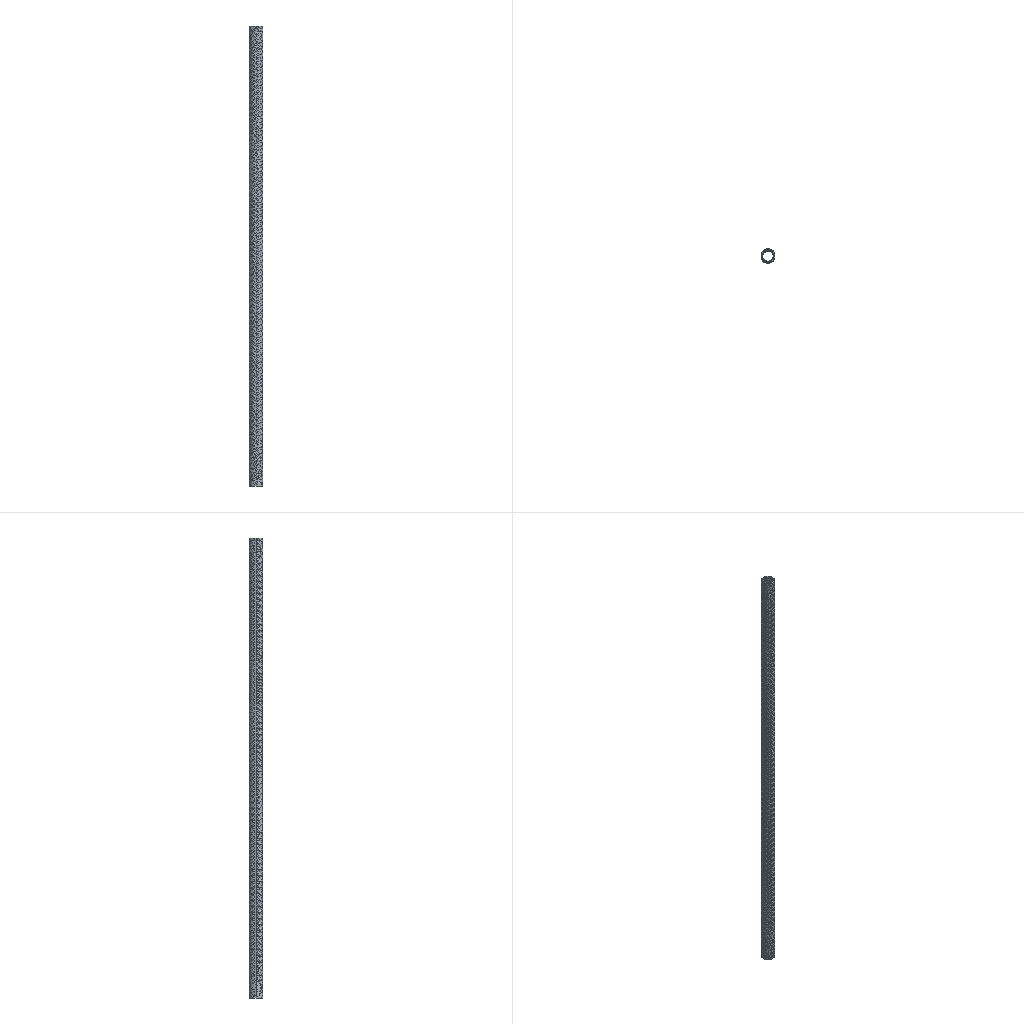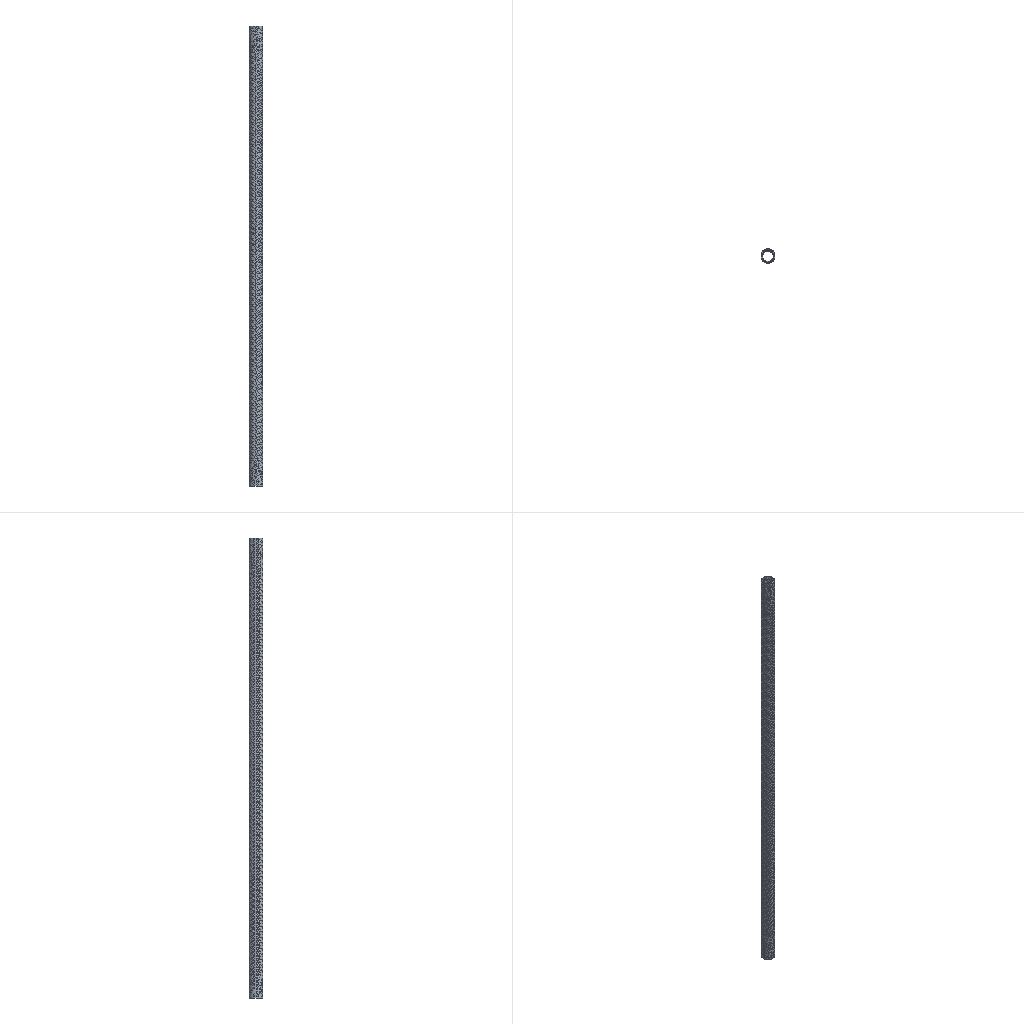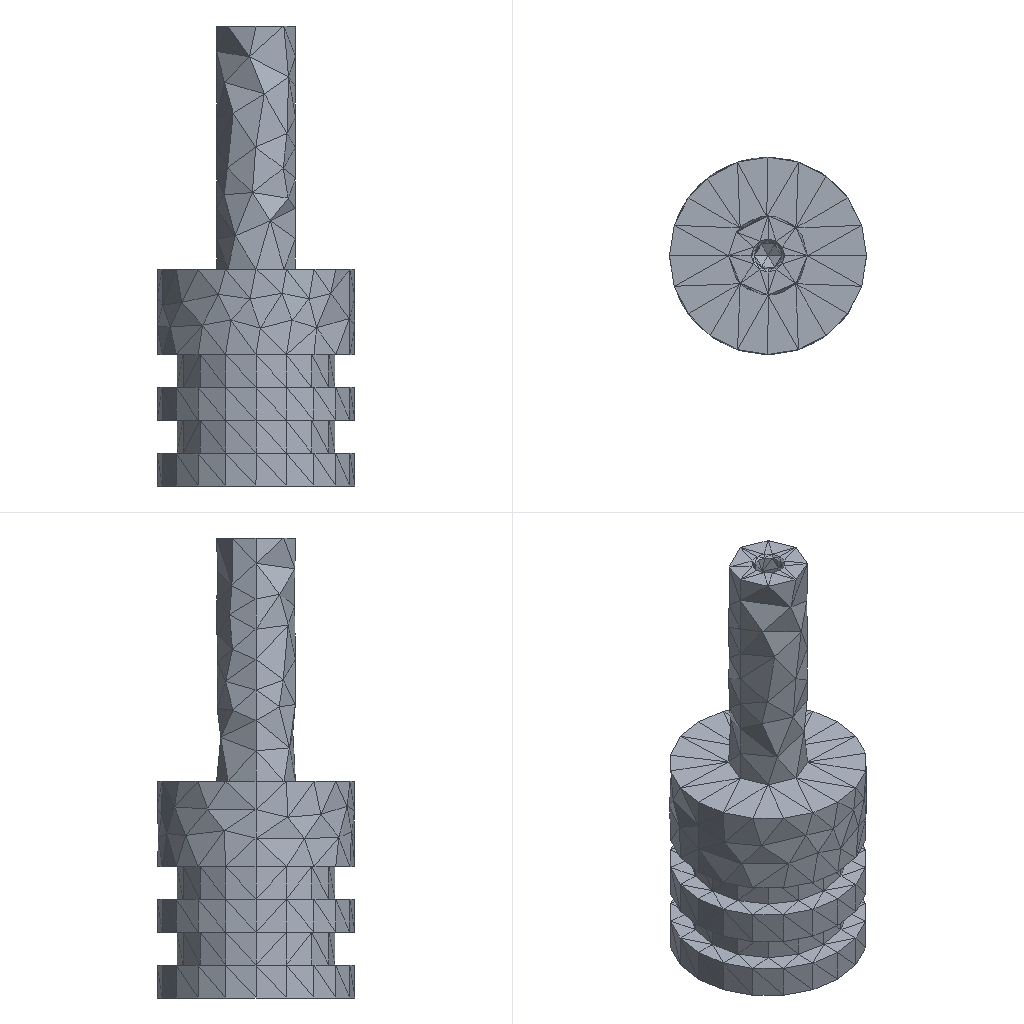Simulation study | ansys workbench
Set-up summary:
category,name,step,type,value,unit,region
solver,ansys_mapdl
solver,version,,,22.1
solver,version,,,22.1
solver,version,,,22.1
solver,version,,,22.1
solver,version,,,22.1
solver,version,,,22.1
units,MPA,,stated
analysis,deck1,,static,static
load_step,requested,,,1
analysis,nlgeom,,,False
mesh,nodes,,,29678
mesh,elements,,,19517
element_type,ANSYS 187 (type 1),,solid,14973
element_type,ANSYS 174 (type 2),,contact,4544
element_type,ANSYS 170 (type 3),,target,0
load,load commands in deck,,count,3
bc,support commands in deck,,count,1
named_set,_FIXEDSU,,component
analysis,deck2,,static,static
load_step,requested,,,1
analysis,nlgeom,,,False
mesh,nodes,,,24907
mesh,elements,,,16520
element_type,ANSYS 187 (type 1),,solid,12612
element_type,ANSYS 174 (type 2),,contact,3908
element_type,ANSYS 170 (type 3),,target,0
load,load commands in deck,,count,3
bc,support commands in deck,,count,1
named_set,_FIXEDSU,,component
analysis,deck3,,static,static
load_step,requested,,,1
analysis,nlgeom,,,False
mesh,nodes,,,2582
mesh,elements,,,1527
element_type,ANSYS 187 (type 1),,solid,1357
element_type,ANSYS 174 (type 2),,contact,170
element_type,ANSYS 170 (type 3),,target,0
load,load commands in deck,,count,3
bc,support commands in deck,,count,1
named_set,_FIXEDSU,,component
analysis,deck4,,static,static
load_step,requested,,,1
analysis,nlgeom,,,False
mesh,nodes,,,1205
mesh,elements,,,665
element_type,ANSYS 187 (type 1),,solid,591
element_type,ANSYS 174 (type 2),,contact,74
element_type,ANSYS 170 (type 3),,target,0
load,load commands in deck,,count,3
bc,support commands in deck,,count,1
named_set,_FIXEDSU,,component
analysis,deck5,,static,static
load_step,requested,,,1
analysis,nlgeom,,,False
mesh,nodes,,,1162
mesh,elements,,,655
element_type,ANSYS 187 (type 1),,solid,567
element_type,ANSYS 174 (type 2),,contact,88
element_type,ANSYS 170 (type 3),,target,0
load,load commands in deck,,count,3
bc,support commands in deck,,count,1
named_set,_FIXEDSU,,component
analysis,deck6,,static,static
load_step,requested,,,1
analysis,nlgeom,,,False
mesh,nodes,,,24907
mesh,elements,,,16520
element_type,ANSYS 187 (type 1),,solid,12612
element_type,ANSYS 174 (type 2),,contact,3908
element_type,ANSYS 170 (type 3),,target,0
load,load commands in deck,,count,3
bc,support commands in deck,,count,1
named_set,_FIXEDSU,,component
material,1,,in results
material,1,,in results
material,1,,in results
material,1,,in results
material,1,,in results
material,1,,in results
check,setup vs results,,match,results also hold 0 node(s) and 1 element(s) the deck makes with ['EN']; those were not compared; 1 node(s) the solver created internally for pilot nodes (ansys-fenxi-1/ansys刀片有限元分析/2222_files/dp0/SYS-1/MECH/solve.out) are in the results only
check,setup vs results,,match,results also hold 0 node(s) and 1 element(s) the deck makes with ['EN']; those were not compared; 1 node(s) the solver created internally for pilot nodes (ansys-fenxi-1/ansys刀片有限元分析/2222_files/dp0/SYS-2/MECH/solve.out) are in the results only
check,setup vs results,,match,results also hold 0 node(s) and 1 element(s) the deck makes with ['EN']; those were not compared; 1 node(s) the solver created internally for pilot nodes (ansys-fenxi-1/ansys刀片有限元分析/2222_files/dp0/SYS-3/MECH/solve.out) are in the results only
check,setup vs results,,match,results also hold 0 node(s) and 1 element(s) the deck makes with ['EN']; those were not compared; 1 node(s) the solver created internally for pilot nodes (ansys-fenxi-1/ansys刀片有限元分析/2222_files/dp0/SYS-4/MECH/solve.out) are in the results only
check,setup vs results,,match,results also hold 0 node(s) and 1 element(s) the deck makes with ['EN']; those were not compared; 1 node(s) the solver created internally for pilot nodes (ansys-fenxi-1/ansys刀片有限元分析/2222_files/dp0/SYS-5/MECH/solve.out) are in the results only
check,setup vs results,,match,results also hold 0 node(s) and 1 element(s) the deck makes with ['EN']; those were not compared; 1 node(s) the solver created internally for pilot nodes (ansys-fenxi-1/ansys刀片有限元分析/2222_files/dp0/SYS/MECH/solve.out) are in the results only
Results summary:
result,analysis,,,static
result,last_loadstep,,,1
result,primary field,,,displacement
result,reaction total,1,FX,-7e-06,N
result,reaction total,1,FY,1e-06,N
result,reaction total,1,FZ,-0.000438,N
result,mass,,,0.0047,"NMM: mm, ton, N, s, mV, mA, degC"
result,analysis,,,static
result,last_loadstep,,,1
result,primary field,,,displacement
result,reaction total,1,FX,7e-06,N
result,reaction total,1,FY,-2e-06,N
result,reaction total,1,FZ,-1.6e-05,N
result,mass,,,0.004744,"NMM: mm, ton, N, s, mV, mA, degC"
result,analysis,,,static
result,last_loadstep,,,1
result,primary field,,,displacement
result,reaction total,1,FX,0.0,N
result,reaction total,1,FY,-0.0,N
result,reaction total,1,FZ,0.0,N
result,mass,,,0.000171,"NMM: mm, ton, N, s, mV, mA, degC"
result,analysis,,,static
result,last_loadstep,,,1
result,primary field,,,displacement
result,reaction total,1,FX,0.0,N
result,reaction total,1,FY,-0.0,N
result,reaction total,1,FZ,-0.0,N
result,mass,,,0.00017,"NMM: mm, ton, N, s, mV, mA, degC"
result,analysis,,,static
result,last_loadstep,,,1
result,primary field,,,displacement
result,reaction total,1,FX,-0.0,N
result,reaction total,1,FY,-0.0,N
result,reaction total,1,FZ,0.0,N
result,mass,,,0.000171,"NMM: mm, ton, N, s, mV, mA, degC"
result,analysis,,,static
result,last_loadstep,,,1
result,primary field,,,displacement
result,reaction total,1,FX,7e-06,N
result,reaction total,1,FY,-2e-06,N
result,reaction total,1,FZ,-1.6e-05,N
result,mass,,,0.004744,"NMM: mm, ton, N, s, mV, mA, degC"